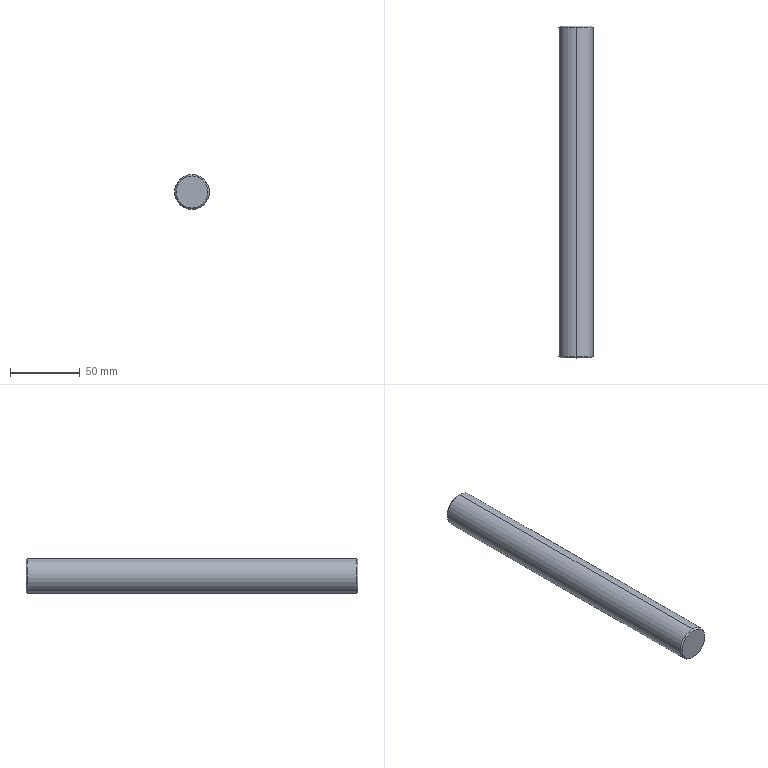Part | STEP file | 012-6-07-018 | 1 solid | 8 faces | box 25 x 238 x 25 mm | volume 116752 mm3 | cone 4 | cylinder 2 | plane 2 | commonest cylinder face diameters 25 x2
STEP:
#1=CARTESIAN_POINT('',(0.,0.,0.));
#2=DIRECTION('',(0.,0.,1.));
#3=DIRECTION('',(1.,0.,0.));
#4=AXIS2_PLACEMENT_3D('',#1,#2,#3);
#5=CARTESIAN_POINT('',(0.,238.,11.5));
#6=VERTEX_POINT('',#5);
#7=CARTESIAN_POINT('',(0.,238.,-11.5));
#8=VERTEX_POINT('',#7);
#9=CARTESIAN_POINT('',(0.,238.,0.));
#10=DIRECTION('',(0.,1.,0.));
#11=DIRECTION('',(0.,0.,1.));
#12=AXIS2_PLACEMENT_3D('',#9,#10,#11);
#13=CIRCLE('',#12,11.5);
#14=CARTESIAN_POINT('',(0.,237.,0.));
#15=DIRECTION('',(0.,-1.,0.));
#16=DIRECTION('',(0.,0.,-1.));
#17=AXIS2_PLACEMENT_3D('',#14,#15,#16);
#18=CONICAL_SURFACE('',#17,12.5,0.7854);
#19=CARTESIAN_POINT('',(3.142,-1.));
#20=DIRECTION('',(-1.,0.));
#21=VECTOR('',#20,1.);
#22=LINE('',#19,#21);
#23=(GEOMETRIC_REPRESENTATION_CONTEXT(2)PARAMETRIC_REPRESENTATION_CONTEXT()REPRESENTATION_CONTEXT('',''));
#24=DEFINITIONAL_REPRESENTATION('',(#22),#23);
#25=PCURVE('',#18,#24);
#26=CARTESIAN_POINT('',(0.,238.,0.));
#27=DIRECTION('',(0.,1.,0.));
#28=DIRECTION('',(0.,0.,1.));
#29=AXIS2_PLACEMENT_3D('',#26,#27,#28);
#30=PLANE('',#29);
#31=CARTESIAN_POINT('',(0.,0.));
#32=DIRECTION('',(1.,0.));
#33=AXIS2_PLACEMENT_2D('',#31,#32);
#34=CIRCLE('',#33,11.5);
#35=(GEOMETRIC_REPRESENTATION_CONTEXT(2)PARAMETRIC_REPRESENTATION_CONTEXT()REPRESENTATION_CONTEXT('',''));
#36=DEFINITIONAL_REPRESENTATION('',(#34),#35);
#37=PCURVE('',#30,#36);
#38=SURFACE_CURVE('',#13,(#25,#37),.PCURVE_S1.);
#39=EDGE_CURVE('',#6,#8,#38,.T.);
#40=ORIENTED_EDGE('',*,*,#39,.F.);
#41=CARTESIAN_POINT('',(0.,237.,12.5));
#42=VERTEX_POINT('',#41);
#43=CARTESIAN_POINT('',(0.,237.,12.5));
#44=DIRECTION('',(0.,-0.7071,0.7071));
#45=VECTOR('',#44,1.);
#46=LINE('',#43,#45);
#47=CARTESIAN_POINT('',(3.142,0.));
#48=DIRECTION('',(0.,1.));
#49=VECTOR('',#48,1.);
#50=LINE('',#47,#49);
#51=(GEOMETRIC_REPRESENTATION_CONTEXT(2)PARAMETRIC_REPRESENTATION_CONTEXT()REPRESENTATION_CONTEXT('',''));
#52=DEFINITIONAL_REPRESENTATION('',(#50),#51);
#53=PCURVE('',#18,#52);
#54=CARTESIAN_POINT('',(0.,237.,0.));
#55=DIRECTION('',(0.,-1.,0.));
#56=DIRECTION('',(0.,0.,-1.));
#57=AXIS2_PLACEMENT_3D('',#54,#55,#56);
#58=CONICAL_SURFACE('',#57,12.5,0.7854);
#59=CARTESIAN_POINT('',(3.142,0.));
#60=DIRECTION('',(0.,1.));
#61=VECTOR('',#60,1.);
#62=LINE('',#59,#61);
#63=(GEOMETRIC_REPRESENTATION_CONTEXT(2)PARAMETRIC_REPRESENTATION_CONTEXT()REPRESENTATION_CONTEXT('',''));
#64=DEFINITIONAL_REPRESENTATION('',(#62),#63);
#65=PCURVE('',#58,#64);
#66=SURFACE_CURVE('',#46,(#53,#65),.PCURVE_S1.);
#67=EDGE_CURVE('',#6,#42,#66,.T.);
#68=ORIENTED_EDGE('',*,*,#67,.T.);
#69=CARTESIAN_POINT('',(0.,237.,-12.5));
#70=VERTEX_POINT('',#69);
#71=CARTESIAN_POINT('',(0.,237.,0.));
#72=DIRECTION('',(0.,-1.,0.));
#73=DIRECTION('',(0.,0.,1.));
#74=AXIS2_PLACEMENT_3D('',#71,#72,#73);
#75=CIRCLE('',#74,12.5);
#76=CARTESIAN_POINT('',(-3.142,0.));
#77=DIRECTION('',(1.,0.));
#78=VECTOR('',#77,1.);
#79=LINE('',#76,#78);
#80=(GEOMETRIC_REPRESENTATION_CONTEXT(2)PARAMETRIC_REPRESENTATION_CONTEXT()REPRESENTATION_CONTEXT('',''));
#81=DEFINITIONAL_REPRESENTATION('',(#79),#80);
#82=PCURVE('',#18,#81);
#83=CARTESIAN_POINT('',(0.,0.,0.));
#84=DIRECTION('',(0.,-1.,0.));
#85=DIRECTION('',(0.,0.,-1.));
#86=AXIS2_PLACEMENT_3D('',#83,#84,#85);
#87=CYLINDRICAL_SURFACE('',#86,12.5);
#88=CARTESIAN_POINT('',(-3.142,-237.));
#89=DIRECTION('',(1.,0.));
#90=VECTOR('',#89,1.);
#91=LINE('',#88,#90);
#92=(GEOMETRIC_REPRESENTATION_CONTEXT(2)PARAMETRIC_REPRESENTATION_CONTEXT()REPRESENTATION_CONTEXT('',''));
#93=DEFINITIONAL_REPRESENTATION('',(#91),#92);
#94=PCURVE('',#87,#93);
#95=SURFACE_CURVE('',#75,(#82,#94),.PCURVE_S1.);
#96=EDGE_CURVE('',#70,#42,#95,.T.);
#97=ORIENTED_EDGE('',*,*,#96,.F.);
#98=CARTESIAN_POINT('',(0.,237.,-12.5));
#99=DIRECTION('',(0.,-0.7071,-0.7071));
#100=VECTOR('',#99,1.);
#101=LINE('',#98,#100);
#102=CARTESIAN_POINT('',(0.,0.));
#103=DIRECTION('',(0.,1.));
#104=VECTOR('',#103,1.);
#105=LINE('',#102,#104);
#106=(GEOMETRIC_REPRESENTATION_CONTEXT(2)PARAMETRIC_REPRESENTATION_CONTEXT()REPRESENTATION_CONTEXT('',''));
#107=DEFINITIONAL_REPRESENTATION('',(#105),#106);
#108=PCURVE('',#18,#107);
#109=CARTESIAN_POINT('',(6.283,0.));
#110=DIRECTION('',(0.,1.));
#111=VECTOR('',#110,1.);
#112=LINE('',#109,#111);
#113=(GEOMETRIC_REPRESENTATION_CONTEXT(2)PARAMETRIC_REPRESENTATION_CONTEXT()REPRESENTATION_CONTEXT('',''));
#114=DEFINITIONAL_REPRESENTATION('',(#112),#113);
#115=PCURVE('',#58,#114);
#116=SURFACE_CURVE('',#101,(#108,#115),.PCURVE_S1.);
#117=EDGE_CURVE('',#8,#70,#116,.T.);
#118=ORIENTED_EDGE('',*,*,#117,.F.);
#119=EDGE_LOOP('',(#40,#68,#97,#118));
#120=FACE_BOUND('',#119,.T.);
#121=ADVANCED_FACE('',(#120),#18,.T.);
#122=CARTESIAN_POINT('',(0.,0.,-11.5));
#123=VERTEX_POINT('',#122);
#124=CARTESIAN_POINT('',(0.,0.,11.5));
#125=VERTEX_POINT('',#124);
#126=CARTESIAN_POINT('',(0.,0.,0.));
#127=DIRECTION('',(0.,-1.,0.));
#128=DIRECTION('',(0.,0.,-1.));
#129=AXIS2_PLACEMENT_3D('',#126,#127,#128);
#130=CIRCLE('',#129,11.5);
#131=CARTESIAN_POINT('',(0.,0.,0.));
#132=DIRECTION('',(0.,1.,0.));
#133=DIRECTION('',(0.,0.,1.));
#134=AXIS2_PLACEMENT_3D('',#131,#132,#133);
#135=CONICAL_SURFACE('',#134,11.5,0.7854);
#136=CARTESIAN_POINT('',(3.142,0.));
#137=DIRECTION('',(-1.,0.));
#138=VECTOR('',#137,1.);
#139=LINE('',#136,#138);
#140=(GEOMETRIC_REPRESENTATION_CONTEXT(2)PARAMETRIC_REPRESENTATION_CONTEXT()REPRESENTATION_CONTEXT('',''));
#141=DEFINITIONAL_REPRESENTATION('',(#139),#140);
#142=PCURVE('',#135,#141);
#143=CARTESIAN_POINT('',(0.,0.,0.));
#144=DIRECTION('',(0.,-1.,0.));
#145=DIRECTION('',(0.,0.,-1.));
#146=AXIS2_PLACEMENT_3D('',#143,#144,#145);
#147=PLANE('',#146);
#148=CARTESIAN_POINT('',(0.,0.));
#149=DIRECTION('',(1.,0.));
#150=AXIS2_PLACEMENT_2D('',#148,#149);
#151=CIRCLE('',#150,11.5);
#152=(GEOMETRIC_REPRESENTATION_CONTEXT(2)PARAMETRIC_REPRESENTATION_CONTEXT()REPRESENTATION_CONTEXT('',''));
#153=DEFINITIONAL_REPRESENTATION('',(#151),#152);
#154=PCURVE('',#147,#153);
#155=SURFACE_CURVE('',#130,(#142,#154),.PCURVE_S1.);
#156=EDGE_CURVE('',#123,#125,#155,.T.);
#157=ORIENTED_EDGE('',*,*,#156,.F.);
#158=CARTESIAN_POINT('',(0.,1.,-12.5));
#159=VERTEX_POINT('',#158);
#160=CARTESIAN_POINT('',(0.,0.,-11.5));
#161=DIRECTION('',(0.,0.7071,-0.7071));
#162=VECTOR('',#161,1.);
#163=LINE('',#160,#162);
#164=CARTESIAN_POINT('',(3.142,0.));
#165=DIRECTION('',(0.,1.));
#166=VECTOR('',#165,1.);
#167=LINE('',#164,#166);
#168=(GEOMETRIC_REPRESENTATION_CONTEXT(2)PARAMETRIC_REPRESENTATION_CONTEXT()REPRESENTATION_CONTEXT('',''));
#169=DEFINITIONAL_REPRESENTATION('',(#167),#168);
#170=PCURVE('',#135,#169);
#171=CARTESIAN_POINT('',(0.,0.,0.));
#172=DIRECTION('',(0.,1.,0.));
#173=DIRECTION('',(0.,0.,1.));
#174=AXIS2_PLACEMENT_3D('',#171,#172,#173);
#175=CONICAL_SURFACE('',#174,11.5,0.7854);
#176=CARTESIAN_POINT('',(3.142,0.));
#177=DIRECTION('',(0.,1.));
#178=VECTOR('',#177,1.);
#179=LINE('',#176,#178);
#180=(GEOMETRIC_REPRESENTATION_CONTEXT(2)PARAMETRIC_REPRESENTATION_CONTEXT()REPRESENTATION_CONTEXT('',''));
#181=DEFINITIONAL_REPRESENTATION('',(#179),#180);
#182=PCURVE('',#175,#181);
#183=SURFACE_CURVE('',#163,(#170,#182),.PCURVE_S1.);
#184=EDGE_CURVE('',#123,#159,#183,.T.);
#185=ORIENTED_EDGE('',*,*,#184,.T.);
#186=CARTESIAN_POINT('',(0.,1.,12.5));
#187=VERTEX_POINT('',#186);
#188=CARTESIAN_POINT('',(0.,1.,0.));
#189=DIRECTION('',(0.,1.,0.));
#190=DIRECTION('',(0.,0.,-1.));
#191=AXIS2_PLACEMENT_3D('',#188,#189,#190);
#192=CIRCLE('',#191,12.5);
#193=CARTESIAN_POINT('',(-3.142,1.));
#194=DIRECTION('',(1.,0.));
#195=VECTOR('',#194,1.);
#196=LINE('',#193,#195);
#197=(GEOMETRIC_REPRESENTATION_CONTEXT(2)PARAMETRIC_REPRESENTATION_CONTEXT()REPRESENTATION_CONTEXT('',''));
#198=DEFINITIONAL_REPRESENTATION('',(#196),#197);
#199=PCURVE('',#135,#198);
#200=CARTESIAN_POINT('',(6.283,-1.));
#201=DIRECTION('',(-1.,0.));
#202=VECTOR('',#201,1.);
#203=LINE('',#200,#202);
#204=(GEOMETRIC_REPRESENTATION_CONTEXT(2)PARAMETRIC_REPRESENTATION_CONTEXT()REPRESENTATION_CONTEXT('',''));
#205=DEFINITIONAL_REPRESENTATION('',(#203),#204);
#206=PCURVE('',#87,#205);
#207=SURFACE_CURVE('',#192,(#199,#206),.PCURVE_S1.);
#208=EDGE_CURVE('',#187,#159,#207,.T.);
#209=ORIENTED_EDGE('',*,*,#208,.F.);
#210=CARTESIAN_POINT('',(0.,0.,11.5));
#211=DIRECTION('',(0.,0.7071,0.7071));
#212=VECTOR('',#211,1.);
#213=LINE('',#210,#212);
#214=CARTESIAN_POINT('',(0.,0.));
#215=DIRECTION('',(0.,1.));
#216=VECTOR('',#215,1.);
#217=LINE('',#214,#216);
#218=(GEOMETRIC_REPRESENTATION_CONTEXT(2)PARAMETRIC_REPRESENTATION_CONTEXT()REPRESENTATION_CONTEXT('',''));
#219=DEFINITIONAL_REPRESENTATION('',(#217),#218);
#220=PCURVE('',#135,#219);
#221=CARTESIAN_POINT('',(6.283,0.));
#222=DIRECTION('',(0.,1.));
#223=VECTOR('',#222,1.);
#224=LINE('',#221,#223);
#225=(GEOMETRIC_REPRESENTATION_CONTEXT(2)PARAMETRIC_REPRESENTATION_CONTEXT()REPRESENTATION_CONTEXT('',''));
#226=DEFINITIONAL_REPRESENTATION('',(#224),#225);
#227=PCURVE('',#175,#226);
#228=SURFACE_CURVE('',#213,(#220,#227),.PCURVE_S1.);
#229=EDGE_CURVE('',#125,#187,#228,.T.);
#230=ORIENTED_EDGE('',*,*,#229,.F.);
#231=EDGE_LOOP('',(#157,#185,#209,#230));
#232=FACE_BOUND('',#231,.T.);
#233=ADVANCED_FACE('',(#232),#135,.T.);
#234=ORIENTED_EDGE('',*,*,#96,.T.);
#235=CARTESIAN_POINT('',(0.,0.,12.5));
#236=DIRECTION('',(0.,-1.,0.));
#237=VECTOR('',#236,1.);
#238=LINE('',#235,#237);
#239=CARTESIAN_POINT('',(3.142,0.));
#240=DIRECTION('',(0.,1.));
#241=VECTOR('',#240,1.);
#242=LINE('',#239,#241);
#243=(GEOMETRIC_REPRESENTATION_CONTEXT(2)PARAMETRIC_REPRESENTATION_CONTEXT()REPRESENTATION_CONTEXT('',''));
#244=DEFINITIONAL_REPRESENTATION('',(#242),#243);
#245=PCURVE('',#87,#244);
#246=CARTESIAN_POINT('',(0.,0.,0.));
#247=DIRECTION('',(0.,-1.,0.));
#248=DIRECTION('',(0.,0.,-1.));
#249=AXIS2_PLACEMENT_3D('',#246,#247,#248);
#250=CYLINDRICAL_SURFACE('',#249,12.5);
#251=CARTESIAN_POINT('',(3.142,0.));
#252=DIRECTION('',(0.,1.));
#253=VECTOR('',#252,1.);
#254=LINE('',#251,#253);
#255=(GEOMETRIC_REPRESENTATION_CONTEXT(2)PARAMETRIC_REPRESENTATION_CONTEXT()REPRESENTATION_CONTEXT('',''));
#256=DEFINITIONAL_REPRESENTATION('',(#254),#255);
#257=PCURVE('',#250,#256);
#258=SURFACE_CURVE('',#238,(#245,#257),.PCURVE_S1.);
#259=EDGE_CURVE('',#42,#187,#258,.T.);
#260=ORIENTED_EDGE('',*,*,#259,.T.);
#261=ORIENTED_EDGE('',*,*,#208,.T.);
#262=CARTESIAN_POINT('',(0.,0.,-12.5));
#263=DIRECTION('',(0.,-1.,0.));
#264=VECTOR('',#263,1.);
#265=LINE('',#262,#264);
#266=CARTESIAN_POINT('',(0.,0.));
#267=DIRECTION('',(0.,1.));
#268=VECTOR('',#267,1.);
#269=LINE('',#266,#268);
#270=(GEOMETRIC_REPRESENTATION_CONTEXT(2)PARAMETRIC_REPRESENTATION_CONTEXT()REPRESENTATION_CONTEXT('',''));
#271=DEFINITIONAL_REPRESENTATION('',(#269),#270);
#272=PCURVE('',#87,#271);
#273=CARTESIAN_POINT('',(6.283,0.));
#274=DIRECTION('',(0.,1.));
#275=VECTOR('',#274,1.);
#276=LINE('',#273,#275);
#277=(GEOMETRIC_REPRESENTATION_CONTEXT(2)PARAMETRIC_REPRESENTATION_CONTEXT()REPRESENTATION_CONTEXT('',''));
#278=DEFINITIONAL_REPRESENTATION('',(#276),#277);
#279=PCURVE('',#250,#278);
#280=SURFACE_CURVE('',#265,(#272,#279),.PCURVE_S1.);
#281=EDGE_CURVE('',#70,#159,#280,.T.);
#282=ORIENTED_EDGE('',*,*,#281,.F.);
#283=EDGE_LOOP('',(#234,#260,#261,#282));
#284=FACE_BOUND('',#283,.T.);
#285=ADVANCED_FACE('',(#284),#87,.T.);
#286=CARTESIAN_POINT('',(0.,238.,0.));
#287=DIRECTION('',(0.,1.,0.));
#288=DIRECTION('',(0.,0.,1.));
#289=AXIS2_PLACEMENT_3D('',#286,#287,#288);
#290=CIRCLE('',#289,11.5);
#291=CARTESIAN_POINT('',(0.,0.));
#292=DIRECTION('',(1.,0.));
#293=AXIS2_PLACEMENT_2D('',#291,#292);
#294=CIRCLE('',#293,11.5);
#295=(GEOMETRIC_REPRESENTATION_CONTEXT(2)PARAMETRIC_REPRESENTATION_CONTEXT()REPRESENTATION_CONTEXT('',''));
#296=DEFINITIONAL_REPRESENTATION('',(#294),#295);
#297=PCURVE('',#30,#296);
#298=CARTESIAN_POINT('',(9.425,-1.));
#299=DIRECTION('',(-1.,0.));
#300=VECTOR('',#299,1.);
#301=LINE('',#298,#300);
#302=(GEOMETRIC_REPRESENTATION_CONTEXT(2)PARAMETRIC_REPRESENTATION_CONTEXT()REPRESENTATION_CONTEXT('',''));
#303=DEFINITIONAL_REPRESENTATION('',(#301),#302);
#304=PCURVE('',#58,#303);
#305=SURFACE_CURVE('',#290,(#297,#304),.PCURVE_S1.);
#306=EDGE_CURVE('',#8,#6,#305,.T.);
#307=ORIENTED_EDGE('',*,*,#306,.T.);
#308=ORIENTED_EDGE('',*,*,#39,.T.);
#309=EDGE_LOOP('',(#307,#308));
#310=FACE_BOUND('',#309,.T.);
#311=ADVANCED_FACE('',(#310),#30,.T.);
#312=ORIENTED_EDGE('',*,*,#259,.F.);
#313=CARTESIAN_POINT('',(0.,237.,0.));
#314=DIRECTION('',(0.,-1.,0.));
#315=DIRECTION('',(0.,0.,1.));
#316=AXIS2_PLACEMENT_3D('',#313,#314,#315);
#317=CIRCLE('',#316,12.5);
#318=CARTESIAN_POINT('',(3.142,-237.));
#319=DIRECTION('',(1.,0.));
#320=VECTOR('',#319,1.);
#321=LINE('',#318,#320);
#322=(GEOMETRIC_REPRESENTATION_CONTEXT(2)PARAMETRIC_REPRESENTATION_CONTEXT()REPRESENTATION_CONTEXT('',''));
#323=DEFINITIONAL_REPRESENTATION('',(#321),#322);
#324=PCURVE('',#250,#323);
#325=CARTESIAN_POINT('',(3.142,0.));
#326=DIRECTION('',(1.,0.));
#327=VECTOR('',#326,1.);
#328=LINE('',#325,#327);
#329=(GEOMETRIC_REPRESENTATION_CONTEXT(2)PARAMETRIC_REPRESENTATION_CONTEXT()REPRESENTATION_CONTEXT('',''));
#330=DEFINITIONAL_REPRESENTATION('',(#328),#329);
#331=PCURVE('',#58,#330);
#332=SURFACE_CURVE('',#317,(#324,#331),.PCURVE_S1.);
#333=EDGE_CURVE('',#42,#70,#332,.T.);
#334=ORIENTED_EDGE('',*,*,#333,.T.);
#335=ORIENTED_EDGE('',*,*,#281,.T.);
#336=CARTESIAN_POINT('',(0.,1.,0.));
#337=DIRECTION('',(0.,1.,0.));
#338=DIRECTION('',(0.,0.,-1.));
#339=AXIS2_PLACEMENT_3D('',#336,#337,#338);
#340=CIRCLE('',#339,12.5);
#341=CARTESIAN_POINT('',(6.283,-1.));
#342=DIRECTION('',(-1.,0.));
#343=VECTOR('',#342,1.);
#344=LINE('',#341,#343);
#345=(GEOMETRIC_REPRESENTATION_CONTEXT(2)PARAMETRIC_REPRESENTATION_CONTEXT()REPRESENTATION_CONTEXT('',''));
#346=DEFINITIONAL_REPRESENTATION('',(#344),#345);
#347=PCURVE('',#250,#346);
#348=CARTESIAN_POINT('',(3.142,1.));
#349=DIRECTION('',(1.,0.));
#350=VECTOR('',#349,1.);
#351=LINE('',#348,#350);
#352=(GEOMETRIC_REPRESENTATION_CONTEXT(2)PARAMETRIC_REPRESENTATION_CONTEXT()REPRESENTATION_CONTEXT('',''));
#353=DEFINITIONAL_REPRESENTATION('',(#351),#352);
#354=PCURVE('',#175,#353);
#355=SURFACE_CURVE('',#340,(#347,#354),.PCURVE_S1.);
#356=EDGE_CURVE('',#159,#187,#355,.T.);
#357=ORIENTED_EDGE('',*,*,#356,.T.);
#358=EDGE_LOOP('',(#312,#334,#335,#357));
#359=FACE_BOUND('',#358,.T.);
#360=ADVANCED_FACE('',(#359),#250,.T.);
#361=CARTESIAN_POINT('',(0.,0.,0.));
#362=DIRECTION('',(0.,-1.,0.));
#363=DIRECTION('',(0.,0.,-1.));
#364=AXIS2_PLACEMENT_3D('',#361,#362,#363);
#365=CIRCLE('',#364,11.5);
#366=CARTESIAN_POINT('',(0.,0.));
#367=DIRECTION('',(1.,0.));
#368=AXIS2_PLACEMENT_2D('',#366,#367);
#369=CIRCLE('',#368,11.5);
#370=(GEOMETRIC_REPRESENTATION_CONTEXT(2)PARAMETRIC_REPRESENTATION_CONTEXT()REPRESENTATION_CONTEXT('',''));
#371=DEFINITIONAL_REPRESENTATION('',(#369),#370);
#372=PCURVE('',#147,#371);
#373=CARTESIAN_POINT('',(9.425,0.));
#374=DIRECTION('',(-1.,0.));
#375=VECTOR('',#374,1.);
#376=LINE('',#373,#375);
#377=(GEOMETRIC_REPRESENTATION_CONTEXT(2)PARAMETRIC_REPRESENTATION_CONTEXT()REPRESENTATION_CONTEXT('',''));
#378=DEFINITIONAL_REPRESENTATION('',(#376),#377);
#379=PCURVE('',#175,#378);
#380=SURFACE_CURVE('',#365,(#372,#379),.PCURVE_S1.);
#381=EDGE_CURVE('',#125,#123,#380,.T.);
#382=ORIENTED_EDGE('',*,*,#381,.T.);
#383=ORIENTED_EDGE('',*,*,#156,.T.);
#384=EDGE_LOOP('',(#382,#383));
#385=FACE_BOUND('',#384,.T.);
#386=ADVANCED_FACE('',(#385),#147,.T.);
#387=ORIENTED_EDGE('',*,*,#184,.F.);
#388=ORIENTED_EDGE('',*,*,#381,.F.);
#389=ORIENTED_EDGE('',*,*,#229,.T.);
#390=ORIENTED_EDGE('',*,*,#356,.F.);
#391=EDGE_LOOP('',(#387,#388,#389,#390));
#392=FACE_BOUND('',#391,.T.);
#393=ADVANCED_FACE('',(#392),#175,.T.);
#394=ORIENTED_EDGE('',*,*,#67,.F.);
#395=ORIENTED_EDGE('',*,*,#306,.F.);
#396=ORIENTED_EDGE('',*,*,#117,.T.);
#397=ORIENTED_EDGE('',*,*,#333,.F.);
#398=EDGE_LOOP('',(#394,#395,#396,#397));
#399=FACE_BOUND('',#398,.T.);
#400=ADVANCED_FACE('',(#399),#58,.T.);
#401=CLOSED_SHELL('',(#121,#233,#285,#311,#360,#386,#393,#400));
#402=MANIFOLD_SOLID_BREP('',#401);
#403=(LENGTH_UNIT()NAMED_UNIT(*)SI_UNIT(.MILLI.,.METRE.));
#404=UNCERTAINTY_MEASURE_WITH_UNIT(LENGTH_MEASURE(0.0000001),#403,'','');
#405=(NAMED_UNIT(*)PLANE_ANGLE_UNIT()SI_UNIT($,.RADIAN.));
#406=(NAMED_UNIT(*)SI_UNIT($,.STERADIAN.)SOLID_ANGLE_UNIT());
#407=(GEOMETRIC_REPRESENTATION_CONTEXT(3)GLOBAL_UNCERTAINTY_ASSIGNED_CONTEXT((#404))GLOBAL_UNIT_ASSIGNED_CONTEXT((#403,#405,#406))REPRESENTATION_CONTEXT('',''));
#408=ADVANCED_BREP_SHAPE_REPRESENTATION('',(#4,#402),#407);